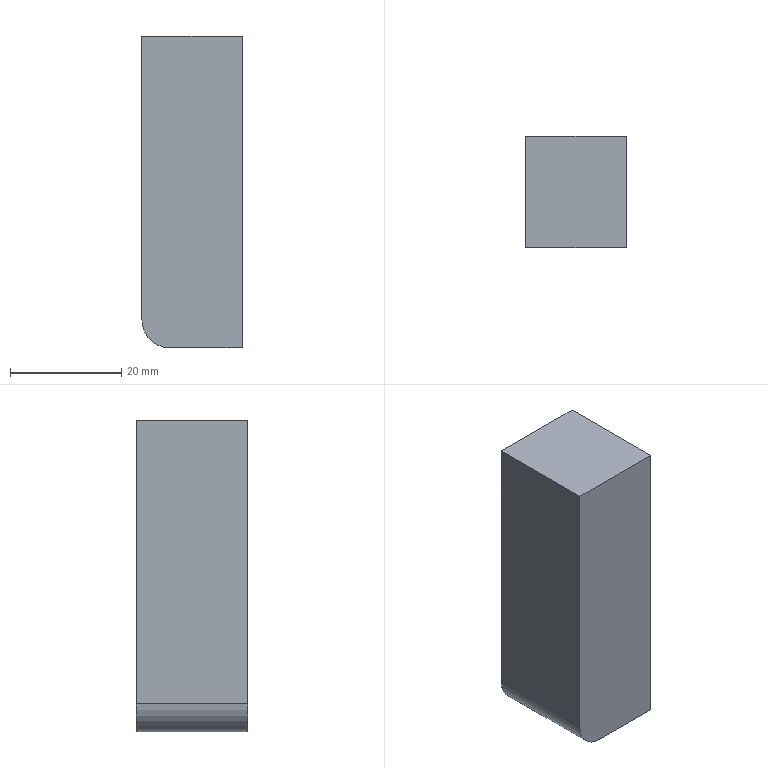Part | STEP file | 1 solid | 7 faces | box 18 x 20 x 56 mm | volume 20053 mm3 | plane 6 | cylinder 1 | commonest cylinder face diameters 10 x1
STEP:
#1=CARTESIAN_POINT('',(0.,0.,0.));
#2=DIRECTION('',(0.,0.,1.));
#3=DIRECTION('',(1.,0.,0.));
#4=AXIS2_PLACEMENT_3D('',#1,#2,#3);
#5=CARTESIAN_POINT('',(-82.862,70.,-36.47));
#6=VERTEX_POINT('',#5);
#7=CARTESIAN_POINT('',(-82.862,50.,-36.47));
#8=VERTEX_POINT('',#7);
#9=CARTESIAN_POINT('',(-82.862,90.366,-36.47));
#10=DIRECTION('',(0.,-1.,0.));
#11=VECTOR('',#10,1.);
#12=LINE('',#9,#11);
#13=CARTESIAN_POINT('',(-72.862,90.366,-36.47));
#14=DIRECTION('',(0.,0.,1.));
#15=DIRECTION('',(1.,0.,0.));
#16=AXIS2_PLACEMENT_3D('',#13,#14,#15);
#17=PLANE('',#16);
#18=CARTESIAN_POINT('',(-10.,0.));
#19=DIRECTION('',(0.,-1.));
#20=VECTOR('',#19,1.);
#21=LINE('',#18,#20);
#22=(GEOMETRIC_REPRESENTATION_CONTEXT(2)PARAMETRIC_REPRESENTATION_CONTEXT()REPRESENTATION_CONTEXT('',''));
#23=DEFINITIONAL_REPRESENTATION('',(#21),#22);
#24=PCURVE('',#17,#23);
#25=CARTESIAN_POINT('',(-82.862,0.,-92.47));
#26=DIRECTION('',(-1.,0.,0.));
#27=DIRECTION('',(0.,0.,1.));
#28=AXIS2_PLACEMENT_3D('',#25,#26,#27);
#29=PLANE('',#28);
#30=CARTESIAN_POINT('',(56.,90.366));
#31=DIRECTION('',(0.,-1.));
#32=VECTOR('',#31,1.);
#33=LINE('',#30,#32);
#34=(GEOMETRIC_REPRESENTATION_CONTEXT(2)PARAMETRIC_REPRESENTATION_CONTEXT()REPRESENTATION_CONTEXT('',''));
#35=DEFINITIONAL_REPRESENTATION('',(#33),#34);
#36=PCURVE('',#29,#35);
#37=SURFACE_CURVE('',#12,(#24,#36),.PCURVE_S1.);
#38=EDGE_CURVE('',#6,#8,#37,.T.);
#39=ORIENTED_EDGE('',*,*,#38,.F.);
#40=CARTESIAN_POINT('',(-100.862,70.,-36.47));
#41=VERTEX_POINT('',#40);
#42=CARTESIAN_POINT('',(-100.862,70.,-36.47));
#43=DIRECTION('',(1.,0.,0.));
#44=VECTOR('',#43,1.);
#45=LINE('',#42,#44);
#46=CARTESIAN_POINT('',(-28.,-20.366));
#47=DIRECTION('',(1.,0.));
#48=VECTOR('',#47,1.);
#49=LINE('',#46,#48);
#50=(GEOMETRIC_REPRESENTATION_CONTEXT(2)PARAMETRIC_REPRESENTATION_CONTEXT()REPRESENTATION_CONTEXT('',''));
#51=DEFINITIONAL_REPRESENTATION('',(#49),#50);
#52=PCURVE('',#17,#51);
#53=CARTESIAN_POINT('',(-100.862,70.,-363.47));
#54=DIRECTION('',(0.,1.,0.));
#55=DIRECTION('',(0.,0.,1.));
#56=AXIS2_PLACEMENT_3D('',#53,#54,#55);
#57=PLANE('',#56);
#58=CARTESIAN_POINT('',(327.,0.));
#59=DIRECTION('',(0.,1.));
#60=VECTOR('',#59,1.);
#61=LINE('',#58,#60);
#62=(GEOMETRIC_REPRESENTATION_CONTEXT(2)PARAMETRIC_REPRESENTATION_CONTEXT()REPRESENTATION_CONTEXT('',''));
#63=DEFINITIONAL_REPRESENTATION('',(#61),#62);
#64=PCURVE('',#57,#63);
#65=SURFACE_CURVE('',#45,(#52,#64),.PCURVE_S1.);
#66=EDGE_CURVE('',#41,#6,#65,.T.);
#67=ORIENTED_EDGE('',*,*,#66,.F.);
#68=CARTESIAN_POINT('',(-100.862,50.,-36.47));
#69=VERTEX_POINT('',#68);
#70=CARTESIAN_POINT('',(-100.862,90.366,-36.47));
#71=DIRECTION('',(0.,-1.,0.));
#72=VECTOR('',#71,1.);
#73=LINE('',#70,#72);
#74=CARTESIAN_POINT('',(-28.,0.));
#75=DIRECTION('',(0.,-1.));
#76=VECTOR('',#75,1.);
#77=LINE('',#74,#76);
#78=(GEOMETRIC_REPRESENTATION_CONTEXT(2)PARAMETRIC_REPRESENTATION_CONTEXT()REPRESENTATION_CONTEXT('',''));
#79=DEFINITIONAL_REPRESENTATION('',(#77),#78);
#80=PCURVE('',#17,#79);
#81=CARTESIAN_POINT('',(-100.862,0.,-92.47));
#82=DIRECTION('',(-1.,0.,0.));
#83=DIRECTION('',(0.,0.,1.));
#84=AXIS2_PLACEMENT_3D('',#81,#82,#83);
#85=PLANE('',#84);
#86=CARTESIAN_POINT('',(56.,90.366));
#87=DIRECTION('',(0.,-1.));
#88=VECTOR('',#87,1.);
#89=LINE('',#86,#88);
#90=(GEOMETRIC_REPRESENTATION_CONTEXT(2)PARAMETRIC_REPRESENTATION_CONTEXT()REPRESENTATION_CONTEXT('',''));
#91=DEFINITIONAL_REPRESENTATION('',(#89),#90);
#92=PCURVE('',#85,#91);
#93=SURFACE_CURVE('',#73,(#80,#92),.PCURVE_S1.);
#94=EDGE_CURVE('',#41,#69,#93,.T.);
#95=ORIENTED_EDGE('',*,*,#94,.T.);
#96=CARTESIAN_POINT('',(-100.862,50.,-36.47));
#97=DIRECTION('',(1.,0.,0.));
#98=VECTOR('',#97,1.);
#99=LINE('',#96,#98);
#100=CARTESIAN_POINT('',(-28.,-40.366));
#101=DIRECTION('',(1.,0.));
#102=VECTOR('',#101,1.);
#103=LINE('',#100,#102);
#104=(GEOMETRIC_REPRESENTATION_CONTEXT(2)PARAMETRIC_REPRESENTATION_CONTEXT()REPRESENTATION_CONTEXT('',''));
#105=DEFINITIONAL_REPRESENTATION('',(#103),#104);
#106=PCURVE('',#17,#105);
#107=CARTESIAN_POINT('',(-100.862,50.,-92.47));
#108=DIRECTION('',(0.,1.,0.));
#109=DIRECTION('',(0.,0.,1.));
#110=AXIS2_PLACEMENT_3D('',#107,#108,#109);
#111=PLANE('',#110);
#112=CARTESIAN_POINT('',(56.,0.));
#113=DIRECTION('',(0.,1.));
#114=VECTOR('',#113,1.);
#115=LINE('',#112,#114);
#116=(GEOMETRIC_REPRESENTATION_CONTEXT(2)PARAMETRIC_REPRESENTATION_CONTEXT()REPRESENTATION_CONTEXT('',''));
#117=DEFINITIONAL_REPRESENTATION('',(#115),#116);
#118=PCURVE('',#111,#117);
#119=SURFACE_CURVE('',#99,(#106,#118),.PCURVE_S1.);
#120=EDGE_CURVE('',#69,#8,#119,.T.);
#121=ORIENTED_EDGE('',*,*,#120,.T.);
#122=EDGE_LOOP('',(#39,#67,#95,#121));
#123=FACE_BOUND('',#122,.T.);
#124=ADVANCED_FACE('',(#123),#17,.T.);
#125=CARTESIAN_POINT('',(-100.862,50.,-87.47));
#126=VERTEX_POINT('',#125);
#127=CARTESIAN_POINT('',(-100.862,50.,-92.47));
#128=DIRECTION('',(0.,0.,1.));
#129=VECTOR('',#128,1.);
#130=LINE('',#127,#129);
#131=CARTESIAN_POINT('',(0.,0.));
#132=DIRECTION('',(1.,0.));
#133=VECTOR('',#132,1.);
#134=LINE('',#131,#133);
#135=(GEOMETRIC_REPRESENTATION_CONTEXT(2)PARAMETRIC_REPRESENTATION_CONTEXT()REPRESENTATION_CONTEXT('',''));
#136=DEFINITIONAL_REPRESENTATION('',(#134),#135);
#137=PCURVE('',#111,#136);
#138=CARTESIAN_POINT('',(0.,50.));
#139=DIRECTION('',(1.,0.));
#140=VECTOR('',#139,1.);
#141=LINE('',#138,#140);
#142=(GEOMETRIC_REPRESENTATION_CONTEXT(2)PARAMETRIC_REPRESENTATION_CONTEXT()REPRESENTATION_CONTEXT('',''));
#143=DEFINITIONAL_REPRESENTATION('',(#141),#142);
#144=PCURVE('',#85,#143);
#145=SURFACE_CURVE('',#130,(#137,#144),.PCURVE_S1.);
#146=EDGE_CURVE('',#126,#69,#145,.T.);
#147=ORIENTED_EDGE('',*,*,#146,.F.);
#148=CARTESIAN_POINT('',(-95.862,50.,-92.47));
#149=VERTEX_POINT('',#148);
#150=CARTESIAN_POINT('',(-95.862,50.,-87.47));
#151=DIRECTION('',(0.,-1.,0.));
#152=DIRECTION('',(0.,0.,1.));
#153=AXIS2_PLACEMENT_3D('',#150,#151,#152);
#154=CIRCLE('',#153,5.);
#155=CARTESIAN_POINT('',(10.,5.));
#156=CARTESIAN_POINT('',(10.,-3.66));
#157=CARTESIAN_POINT('',(2.5,0.6699));
#158=CARTESIAN_POINT('',(-5.,5.));
#159=CARTESIAN_POINT('',(2.5,9.33));
#160=CARTESIAN_POINT('',(10.,13.66));
#161=CARTESIAN_POINT('',(10.,5.));
#162=(BOUNDED_CURVE()B_SPLINE_CURVE(2,(#155,#156,#157,#158,#159,#160,#161),.UNSPECIFIED.,.T.,.F.)B_SPLINE_CURVE_WITH_KNOTS((1,2,2,2,2,1),(-2.094,0.,2.094,4.189,6.283,8.378),.UNSPECIFIED.)CURVE()GEOMETRIC_REPRESENTATION_ITEM()RATIONAL_B_SPLINE_CURVE((1.,0.5,1.,0.5,1.,0.5,1.))REPRESENTATION_ITEM(''));
#163=(GEOMETRIC_REPRESENTATION_CONTEXT(2)PARAMETRIC_REPRESENTATION_CONTEXT()REPRESENTATION_CONTEXT('',''));
#164=DEFINITIONAL_REPRESENTATION('',(#162),#163);
#165=PCURVE('',#111,#164);
#166=CARTESIAN_POINT('',(-95.862,0.,-87.47));
#167=DIRECTION('',(0.,1.,0.));
#168=DIRECTION('',(0.,0.,1.));
#169=AXIS2_PLACEMENT_3D('',#166,#167,#168);
#170=CYLINDRICAL_SURFACE('',#169,5.);
#171=CARTESIAN_POINT('',(6.283,50.));
#172=DIRECTION('',(-1.,0.));
#173=VECTOR('',#172,1.);
#174=LINE('',#171,#173);
#175=(GEOMETRIC_REPRESENTATION_CONTEXT(2)PARAMETRIC_REPRESENTATION_CONTEXT()REPRESENTATION_CONTEXT('',''));
#176=DEFINITIONAL_REPRESENTATION('',(#174),#175);
#177=PCURVE('',#170,#176);
#178=SURFACE_CURVE('',#154,(#165,#177),.PCURVE_S1.);
#179=EDGE_CURVE('',#126,#149,#178,.T.);
#180=ORIENTED_EDGE('',*,*,#179,.T.);
#181=CARTESIAN_POINT('',(-82.862,50.,-92.47));
#182=VERTEX_POINT('',#181);
#183=CARTESIAN_POINT('',(-95.862,50.,-92.47));
#184=CARTESIAN_POINT('',(-91.529,50.,-92.47));
#185=CARTESIAN_POINT('',(-87.196,50.,-92.47));
#186=CARTESIAN_POINT('',(-82.862,50.,-92.47));
#187=B_SPLINE_CURVE_WITH_KNOTS('',3,(#183,#184,#185,#186),.UNSPECIFIED.,.F.,.F.,(4,4),(0.2778,1.),.PIECEWISE_BEZIER_KNOTS.);
#188=CARTESIAN_POINT('',(0.,5.));
#189=CARTESIAN_POINT('',(0.,9.333));
#190=CARTESIAN_POINT('',(0.,13.667));
#191=CARTESIAN_POINT('',(0.,18.));
#192=B_SPLINE_CURVE_WITH_KNOTS('',3,(#188,#189,#190,#191),.UNSPECIFIED.,.F.,.F.,(4,4),(0.2778,1.),.PIECEWISE_BEZIER_KNOTS.);
#193=(GEOMETRIC_REPRESENTATION_CONTEXT(2)PARAMETRIC_REPRESENTATION_CONTEXT()REPRESENTATION_CONTEXT('',''));
#194=DEFINITIONAL_REPRESENTATION('',(#192),#193);
#195=PCURVE('',#111,#194);
#196=CARTESIAN_POINT('',(-100.862,0.,-92.47));
#197=DIRECTION('',(0.,0.,1.));
#198=DIRECTION('',(1.,0.,0.));
#199=AXIS2_PLACEMENT_3D('',#196,#197,#198);
#200=PLANE('',#199);
#201=CARTESIAN_POINT('',(5.,50.));
#202=CARTESIAN_POINT('',(9.333,50.));
#203=CARTESIAN_POINT('',(13.667,50.));
#204=CARTESIAN_POINT('',(18.,50.));
#205=B_SPLINE_CURVE_WITH_KNOTS('',3,(#201,#202,#203,#204),.UNSPECIFIED.,.F.,.F.,(4,4),(0.2778,1.),.PIECEWISE_BEZIER_KNOTS.);
#206=(GEOMETRIC_REPRESENTATION_CONTEXT(2)PARAMETRIC_REPRESENTATION_CONTEXT()REPRESENTATION_CONTEXT('',''));
#207=DEFINITIONAL_REPRESENTATION('',(#205),#206);
#208=PCURVE('',#200,#207);
#209=SURFACE_CURVE('',#187,(#195,#208),.PCURVE_S1.);
#210=EDGE_CURVE('',#149,#182,#209,.T.);
#211=ORIENTED_EDGE('',*,*,#210,.T.);
#212=CARTESIAN_POINT('',(-82.862,50.,-92.47));
#213=DIRECTION('',(0.,0.,1.));
#214=VECTOR('',#213,1.);
#215=LINE('',#212,#214);
#216=CARTESIAN_POINT('',(0.,18.));
#217=DIRECTION('',(1.,0.));
#218=VECTOR('',#217,1.);
#219=LINE('',#216,#218);
#220=(GEOMETRIC_REPRESENTATION_CONTEXT(2)PARAMETRIC_REPRESENTATION_CONTEXT()REPRESENTATION_CONTEXT('',''));
#221=DEFINITIONAL_REPRESENTATION('',(#219),#220);
#222=PCURVE('',#111,#221);
#223=CARTESIAN_POINT('',(0.,50.));
#224=DIRECTION('',(1.,0.));
#225=VECTOR('',#224,1.);
#226=LINE('',#223,#225);
#227=(GEOMETRIC_REPRESENTATION_CONTEXT(2)PARAMETRIC_REPRESENTATION_CONTEXT()REPRESENTATION_CONTEXT('',''));
#228=DEFINITIONAL_REPRESENTATION('',(#226),#227);
#229=PCURVE('',#29,#228);
#230=SURFACE_CURVE('',#215,(#222,#229),.PCURVE_S1.);
#231=EDGE_CURVE('',#182,#8,#230,.T.);
#232=ORIENTED_EDGE('',*,*,#231,.T.);
#233=ORIENTED_EDGE('',*,*,#120,.F.);
#234=EDGE_LOOP('',(#147,#180,#211,#232,#233));
#235=FACE_BOUND('',#234,.T.);
#236=ADVANCED_FACE('',(#235),#111,.F.);
#237=ORIENTED_EDGE('',*,*,#210,.F.);
#238=CARTESIAN_POINT('',(-95.862,70.,-92.47));
#239=VERTEX_POINT('',#238);
#240=CARTESIAN_POINT('',(-95.862,70.,-92.47));
#241=DIRECTION('',(0.,1.,0.));
#242=VECTOR('',#241,1.);
#243=LINE('',#240,#242);
#244=CARTESIAN_POINT('',(5.,70.));
#245=DIRECTION('',(0.,1.));
#246=VECTOR('',#245,1.);
#247=LINE('',#244,#246);
#248=(GEOMETRIC_REPRESENTATION_CONTEXT(2)PARAMETRIC_REPRESENTATION_CONTEXT()REPRESENTATION_CONTEXT('',''));
#249=DEFINITIONAL_REPRESENTATION('',(#247),#248);
#250=PCURVE('',#200,#249);
#251=CARTESIAN_POINT('',(3.142,70.));
#252=DIRECTION('',(0.,1.));
#253=VECTOR('',#252,1.);
#254=LINE('',#251,#253);
#255=(GEOMETRIC_REPRESENTATION_CONTEXT(2)PARAMETRIC_REPRESENTATION_CONTEXT()REPRESENTATION_CONTEXT('',''));
#256=DEFINITIONAL_REPRESENTATION('',(#254),#255);
#257=PCURVE('',#170,#256);
#258=SURFACE_CURVE('',#243,(#250,#257),.PCURVE_S1.);
#259=EDGE_CURVE('',#149,#239,#258,.T.);
#260=ORIENTED_EDGE('',*,*,#259,.T.);
#261=CARTESIAN_POINT('',(-82.862,70.,-92.47));
#262=VERTEX_POINT('',#261);
#263=CARTESIAN_POINT('',(-100.862,70.,-92.47));
#264=DIRECTION('',(1.,0.,0.));
#265=VECTOR('',#264,1.);
#266=LINE('',#263,#265);
#267=CARTESIAN_POINT('',(0.,70.));
#268=DIRECTION('',(1.,0.));
#269=VECTOR('',#268,1.);
#270=LINE('',#267,#269);
#271=(GEOMETRIC_REPRESENTATION_CONTEXT(2)PARAMETRIC_REPRESENTATION_CONTEXT()REPRESENTATION_CONTEXT('',''));
#272=DEFINITIONAL_REPRESENTATION('',(#270),#271);
#273=PCURVE('',#200,#272);
#274=CARTESIAN_POINT('',(271.,0.));
#275=DIRECTION('',(0.,1.));
#276=VECTOR('',#275,1.);
#277=LINE('',#274,#276);
#278=(GEOMETRIC_REPRESENTATION_CONTEXT(2)PARAMETRIC_REPRESENTATION_CONTEXT()REPRESENTATION_CONTEXT('',''));
#279=DEFINITIONAL_REPRESENTATION('',(#277),#278);
#280=PCURVE('',#57,#279);
#281=SURFACE_CURVE('',#266,(#273,#280),.PCURVE_S1.);
#282=EDGE_CURVE('',#239,#262,#281,.T.);
#283=ORIENTED_EDGE('',*,*,#282,.T.);
#284=CARTESIAN_POINT('',(-82.862,0.,-92.47));
#285=DIRECTION('',(0.,-1.,0.));
#286=VECTOR('',#285,1.);
#287=LINE('',#284,#286);
#288=CARTESIAN_POINT('',(18.,0.));
#289=DIRECTION('',(0.,-1.));
#290=VECTOR('',#289,1.);
#291=LINE('',#288,#290);
#292=(GEOMETRIC_REPRESENTATION_CONTEXT(2)PARAMETRIC_REPRESENTATION_CONTEXT()REPRESENTATION_CONTEXT('',''));
#293=DEFINITIONAL_REPRESENTATION('',(#291),#292);
#294=PCURVE('',#200,#293);
#295=CARTESIAN_POINT('',(0.,0.));
#296=DIRECTION('',(0.,-1.));
#297=VECTOR('',#296,1.);
#298=LINE('',#295,#297);
#299=(GEOMETRIC_REPRESENTATION_CONTEXT(2)PARAMETRIC_REPRESENTATION_CONTEXT()REPRESENTATION_CONTEXT('',''));
#300=DEFINITIONAL_REPRESENTATION('',(#298),#299);
#301=PCURVE('',#29,#300);
#302=SURFACE_CURVE('',#287,(#294,#301),.PCURVE_S1.);
#303=EDGE_CURVE('',#262,#182,#302,.T.);
#304=ORIENTED_EDGE('',*,*,#303,.T.);
#305=EDGE_LOOP('',(#237,#260,#283,#304));
#306=FACE_BOUND('',#305,.T.);
#307=ADVANCED_FACE('',(#306),#200,.F.);
#308=ORIENTED_EDGE('',*,*,#282,.F.);
#309=CARTESIAN_POINT('',(-100.862,70.,-87.47));
#310=VERTEX_POINT('',#309);
#311=CARTESIAN_POINT('',(-95.862,70.,-87.47));
#312=DIRECTION('',(0.,1.,0.));
#313=DIRECTION('',(0.,0.,1.));
#314=AXIS2_PLACEMENT_3D('',#311,#312,#313);
#315=CIRCLE('',#314,5.);
#316=CARTESIAN_POINT('',(276.,5.));
#317=DIRECTION('',(1.,0.));
#318=AXIS2_PLACEMENT_2D('',#316,#317);
#319=CIRCLE('',#318,5.);
#320=(GEOMETRIC_REPRESENTATION_CONTEXT(2)PARAMETRIC_REPRESENTATION_CONTEXT()REPRESENTATION_CONTEXT('',''));
#321=DEFINITIONAL_REPRESENTATION('',(#319),#320);
#322=PCURVE('',#57,#321);
#323=CARTESIAN_POINT('',(0.,70.));
#324=DIRECTION('',(1.,0.));
#325=VECTOR('',#324,1.);
#326=LINE('',#323,#325);
#327=(GEOMETRIC_REPRESENTATION_CONTEXT(2)PARAMETRIC_REPRESENTATION_CONTEXT()REPRESENTATION_CONTEXT('',''));
#328=DEFINITIONAL_REPRESENTATION('',(#326),#327);
#329=PCURVE('',#170,#328);
#330=SURFACE_CURVE('',#315,(#322,#329),.PCURVE_S1.);
#331=EDGE_CURVE('',#239,#310,#330,.T.);
#332=ORIENTED_EDGE('',*,*,#331,.T.);
#333=CARTESIAN_POINT('',(-100.862,70.,-363.47));
#334=DIRECTION('',(0.,0.,1.));
#335=VECTOR('',#334,1.);
#336=LINE('',#333,#335);
#337=CARTESIAN_POINT('',(0.,0.));
#338=DIRECTION('',(1.,0.));
#339=VECTOR('',#338,1.);
#340=LINE('',#337,#339);
#341=(GEOMETRIC_REPRESENTATION_CONTEXT(2)PARAMETRIC_REPRESENTATION_CONTEXT()REPRESENTATION_CONTEXT('',''));
#342=DEFINITIONAL_REPRESENTATION('',(#340),#341);
#343=PCURVE('',#57,#342);
#344=CARTESIAN_POINT('',(-271.,70.));
#345=DIRECTION('',(1.,0.));
#346=VECTOR('',#345,1.);
#347=LINE('',#344,#346);
#348=(GEOMETRIC_REPRESENTATION_CONTEXT(2)PARAMETRIC_REPRESENTATION_CONTEXT()REPRESENTATION_CONTEXT('',''));
#349=DEFINITIONAL_REPRESENTATION('',(#347),#348);
#350=PCURVE('',#85,#349);
#351=SURFACE_CURVE('',#336,(#343,#350),.PCURVE_S1.);
#352=EDGE_CURVE('',#310,#41,#351,.T.);
#353=ORIENTED_EDGE('',*,*,#352,.T.);
#354=ORIENTED_EDGE('',*,*,#66,.T.);
#355=CARTESIAN_POINT('',(-82.862,70.,-363.47));
#356=DIRECTION('',(0.,0.,1.));
#357=VECTOR('',#356,1.);
#358=LINE('',#355,#357);
#359=CARTESIAN_POINT('',(0.,18.));
#360=DIRECTION('',(1.,0.));
#361=VECTOR('',#360,1.);
#362=LINE('',#359,#361);
#363=(GEOMETRIC_REPRESENTATION_CONTEXT(2)PARAMETRIC_REPRESENTATION_CONTEXT()REPRESENTATION_CONTEXT('',''));
#364=DEFINITIONAL_REPRESENTATION('',(#362),#363);
#365=PCURVE('',#57,#364);
#366=CARTESIAN_POINT('',(-271.,70.));
#367=DIRECTION('',(1.,0.));
#368=VECTOR('',#367,1.);
#369=LINE('',#366,#368);
#370=(GEOMETRIC_REPRESENTATION_CONTEXT(2)PARAMETRIC_REPRESENTATION_CONTEXT()REPRESENTATION_CONTEXT('',''));
#371=DEFINITIONAL_REPRESENTATION('',(#369),#370);
#372=PCURVE('',#29,#371);
#373=SURFACE_CURVE('',#358,(#365,#372),.PCURVE_S1.);
#374=EDGE_CURVE('',#262,#6,#373,.T.);
#375=ORIENTED_EDGE('',*,*,#374,.F.);
#376=EDGE_LOOP('',(#308,#332,#353,#354,#375));
#377=FACE_BOUND('',#376,.T.);
#378=ADVANCED_FACE('',(#377),#57,.T.);
#379=ORIENTED_EDGE('',*,*,#352,.F.);
#380=CARTESIAN_POINT('',(-100.862,50.,-87.47));
#381=DIRECTION('',(0.,-1.,0.));
#382=VECTOR('',#381,1.);
#383=LINE('',#380,#382);
#384=CARTESIAN_POINT('',(5.,50.));
#385=DIRECTION('',(0.,-1.));
#386=VECTOR('',#385,1.);
#387=LINE('',#384,#386);
#388=(GEOMETRIC_REPRESENTATION_CONTEXT(2)PARAMETRIC_REPRESENTATION_CONTEXT()REPRESENTATION_CONTEXT('',''));
#389=DEFINITIONAL_REPRESENTATION('',(#387),#388);
#390=PCURVE('',#85,#389);
#391=CARTESIAN_POINT('',(4.712,50.));
#392=DIRECTION('',(0.,-1.));
#393=VECTOR('',#392,1.);
#394=LINE('',#391,#393);
#395=(GEOMETRIC_REPRESENTATION_CONTEXT(2)PARAMETRIC_REPRESENTATION_CONTEXT()REPRESENTATION_CONTEXT('',''));
#396=DEFINITIONAL_REPRESENTATION('',(#394),#395);
#397=PCURVE('',#170,#396);
#398=SURFACE_CURVE('',#383,(#390,#397),.PCURVE_S1.);
#399=EDGE_CURVE('',#310,#126,#398,.T.);
#400=ORIENTED_EDGE('',*,*,#399,.T.);
#401=ORIENTED_EDGE('',*,*,#146,.T.);
#402=ORIENTED_EDGE('',*,*,#94,.F.);
#403=EDGE_LOOP('',(#379,#400,#401,#402));
#404=FACE_BOUND('',#403,.T.);
#405=ADVANCED_FACE('',(#404),#85,.T.);
#406=ORIENTED_EDGE('',*,*,#38,.T.);
#407=ORIENTED_EDGE('',*,*,#231,.F.);
#408=ORIENTED_EDGE('',*,*,#303,.F.);
#409=ORIENTED_EDGE('',*,*,#374,.T.);
#410=EDGE_LOOP('',(#406,#407,#408,#409));
#411=FACE_BOUND('',#410,.T.);
#412=ADVANCED_FACE('',(#411),#29,.F.);
#413=ORIENTED_EDGE('',*,*,#331,.F.);
#414=ORIENTED_EDGE('',*,*,#259,.F.);
#415=ORIENTED_EDGE('',*,*,#179,.F.);
#416=ORIENTED_EDGE('',*,*,#399,.F.);
#417=EDGE_LOOP('',(#413,#414,#415,#416));
#418=FACE_BOUND('',#417,.T.);
#419=ADVANCED_FACE('',(#418),#170,.T.);
#420=CLOSED_SHELL('',(#124,#236,#307,#378,#405,#412,#419));
#421=MANIFOLD_SOLID_BREP('',#420);
#422=(LENGTH_UNIT()NAMED_UNIT(*)SI_UNIT(.MILLI.,.METRE.));
#423=UNCERTAINTY_MEASURE_WITH_UNIT(LENGTH_MEASURE(0.0000001),#422,'','');
#424=(NAMED_UNIT(*)PLANE_ANGLE_UNIT()SI_UNIT($,.RADIAN.));
#425=(NAMED_UNIT(*)SI_UNIT($,.STERADIAN.)SOLID_ANGLE_UNIT());
#426=(GEOMETRIC_REPRESENTATION_CONTEXT(3)GLOBAL_UNCERTAINTY_ASSIGNED_CONTEXT((#423))GLOBAL_UNIT_ASSIGNED_CONTEXT((#422,#424,#425))REPRESENTATION_CONTEXT('',''));
#427=ADVANCED_BREP_SHAPE_REPRESENTATION('',(#4,#421),#426);